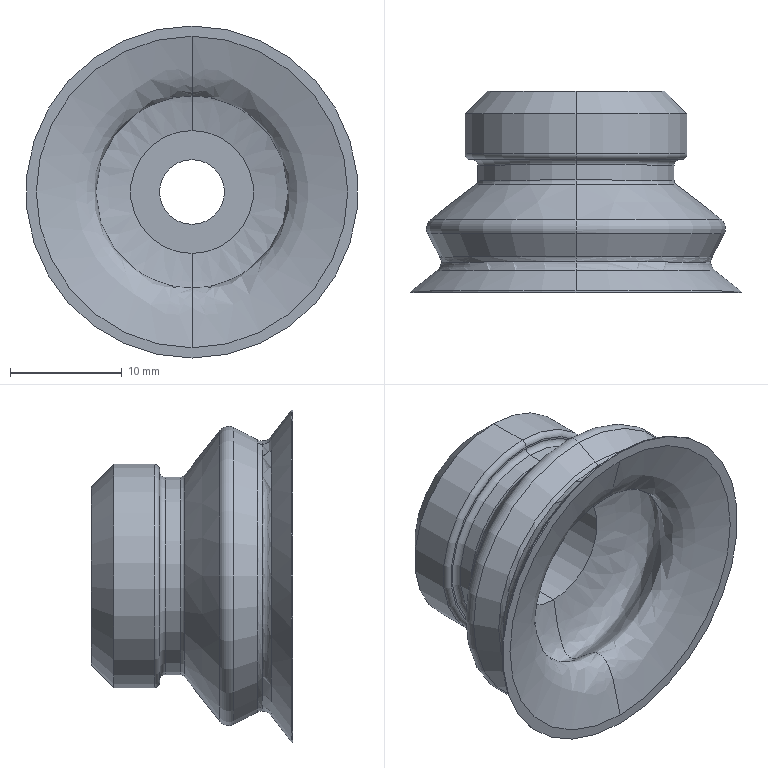Part | STEP file | PJG-30 | 1 solid | 36 faces | box 29.715 x 18 x 29.715 mm | volume 4013 mm3 | torus 12 | cone 10 | cylinder 8 | plane 4 | spline 2 | commonest cylinder face diameters 5.8 x2 11 x2 17.676 x2 20 x2